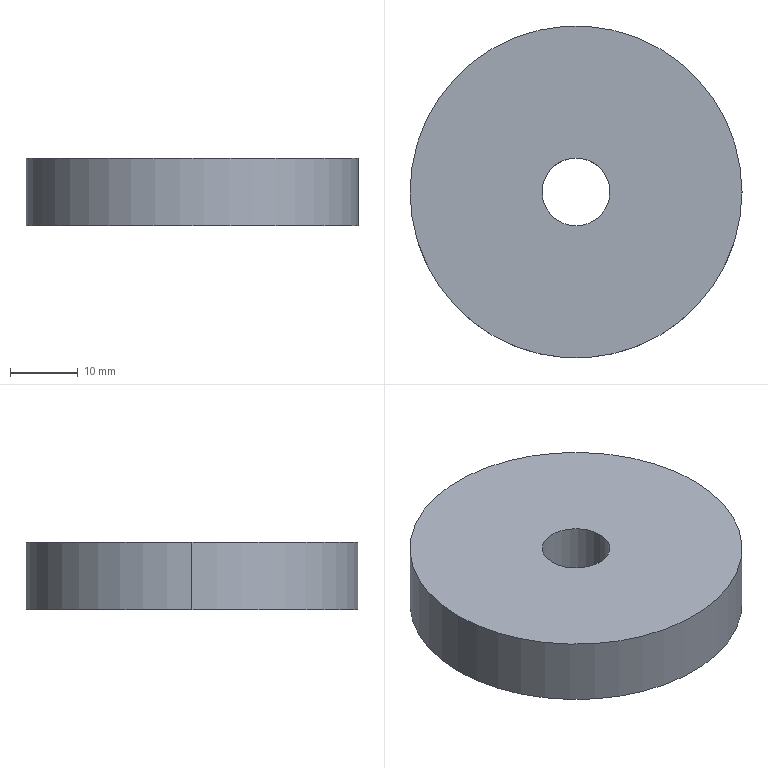Part | STEP file | Produce dryer HY-40-M-bushing clamp plate | 1 solid | 6 faces | box 49 x 49 x 10 mm | volume 18072 mm3 | cylinder 4 | plane 2 | commonest cylinder face diameters 10 x2 49 x2
STEP:
#1=CARTESIAN_POINT('',(-5.,0.,10.));
#2=VERTEX_POINT('',#1);
#3=CARTESIAN_POINT('',(5.,0.,10.));
#4=VERTEX_POINT('',#3);
#5=CARTESIAN_POINT('',(0.,0.,10.));
#6=DIRECTION('',(0.,0.,1.));
#7=DIRECTION('',(1.,0.,0.));
#8=AXIS2_PLACEMENT_3D('',#5,#6,#7);
#9=CIRCLE('',#8,5.);
#10=EDGE_CURVE('',#2,#4,#9,.T.);
#11=ORIENTED_EDGE('',*,*,#10,.T.);
#12=CARTESIAN_POINT('',(5.,0.,0.));
#13=VERTEX_POINT('',#12);
#14=CARTESIAN_POINT('',(5.,0.,10.));
#15=DIRECTION('',(0.,0.,-1.));
#16=VECTOR('',#15,1000.);
#17=LINE('',#14,#16);
#18=EDGE_CURVE('',#4,#13,#17,.T.);
#19=ORIENTED_EDGE('',*,*,#18,.T.);
#20=CARTESIAN_POINT('',(-5.,0.,0.));
#21=VERTEX_POINT('',#20);
#22=CARTESIAN_POINT('',(0.,0.,0.));
#23=DIRECTION('',(0.,0.,1.));
#24=DIRECTION('',(1.,0.,0.));
#25=AXIS2_PLACEMENT_3D('',#22,#23,#24);
#26=CIRCLE('',#25,5.);
#27=EDGE_CURVE('',#21,#13,#26,.T.);
#28=ORIENTED_EDGE('',*,*,#27,.F.);
#29=CARTESIAN_POINT('',(-5.,0.,10.));
#30=DIRECTION('',(0.,0.,-1.));
#31=VECTOR('',#30,1000.);
#32=LINE('',#29,#31);
#33=EDGE_CURVE('',#2,#21,#32,.T.);
#34=ORIENTED_EDGE('',*,*,#33,.F.);
#35=EDGE_LOOP('',(#11,#19,#28,#34));
#36=FACE_OUTER_BOUND('',#35,.T.);
#37=CARTESIAN_POINT('',(0.,0.,10.));
#38=DIRECTION('',(0.,0.,-1.));
#39=DIRECTION('',(-1.,0.,0.));
#40=AXIS2_PLACEMENT_3D('',#37,#38,#39);
#41=CYLINDRICAL_SURFACE('',#40,5.);
#42=ADVANCED_FACE('',(#36),#41,.F.);
#43=CARTESIAN_POINT('',(24.5,0.,10.));
#44=VERTEX_POINT('',#43);
#45=CARTESIAN_POINT('',(-24.5,0.,10.));
#46=VERTEX_POINT('',#45);
#47=CARTESIAN_POINT('',(0.,0.,10.));
#48=DIRECTION('',(0.,0.,1.));
#49=DIRECTION('',(1.,0.,0.));
#50=AXIS2_PLACEMENT_3D('',#47,#48,#49);
#51=CIRCLE('',#50,24.5);
#52=EDGE_CURVE('',#44,#46,#51,.T.);
#53=ORIENTED_EDGE('',*,*,#52,.F.);
#54=CARTESIAN_POINT('',(24.5,0.,0.));
#55=VERTEX_POINT('',#54);
#56=CARTESIAN_POINT('',(24.5,0.,10.));
#57=DIRECTION('',(0.,0.,-1.));
#58=VECTOR('',#57,1000.);
#59=LINE('',#56,#58);
#60=EDGE_CURVE('',#44,#55,#59,.T.);
#61=ORIENTED_EDGE('',*,*,#60,.T.);
#62=CARTESIAN_POINT('',(-24.5,0.,0.));
#63=VERTEX_POINT('',#62);
#64=CARTESIAN_POINT('',(0.,0.,0.));
#65=DIRECTION('',(0.,0.,1.));
#66=DIRECTION('',(1.,0.,0.));
#67=AXIS2_PLACEMENT_3D('',#64,#65,#66);
#68=CIRCLE('',#67,24.5);
#69=EDGE_CURVE('',#55,#63,#68,.T.);
#70=ORIENTED_EDGE('',*,*,#69,.T.);
#71=CARTESIAN_POINT('',(-24.5,0.,10.));
#72=DIRECTION('',(0.,0.,-1.));
#73=VECTOR('',#72,1000.);
#74=LINE('',#71,#73);
#75=EDGE_CURVE('',#46,#63,#74,.T.);
#76=ORIENTED_EDGE('',*,*,#75,.F.);
#77=EDGE_LOOP('',(#53,#61,#70,#76));
#78=FACE_OUTER_BOUND('',#77,.T.);
#79=CARTESIAN_POINT('',(0.,0.,10.));
#80=DIRECTION('',(0.,0.,-1.));
#81=DIRECTION('',(-1.,0.,0.));
#82=AXIS2_PLACEMENT_3D('',#79,#80,#81);
#83=CYLINDRICAL_SURFACE('',#82,24.5);
#84=ADVANCED_FACE('',(#78),#83,.T.);
#85=CARTESIAN_POINT('',(0.,0.,10.));
#86=DIRECTION('',(0.,0.,1.));
#87=DIRECTION('',(1.,0.,0.));
#88=AXIS2_PLACEMENT_3D('',#85,#86,#87);
#89=CIRCLE('',#88,24.5);
#90=EDGE_CURVE('',#46,#44,#89,.T.);
#91=ORIENTED_EDGE('',*,*,#90,.T.);
#92=ORIENTED_EDGE('',*,*,#52,.T.);
#93=EDGE_LOOP('',(#91,#92));
#94=FACE_OUTER_BOUND('',#93,.T.);
#95=ORIENTED_EDGE('',*,*,#10,.F.);
#96=CARTESIAN_POINT('',(0.,0.,10.));
#97=DIRECTION('',(0.,0.,1.));
#98=DIRECTION('',(1.,0.,0.));
#99=AXIS2_PLACEMENT_3D('',#96,#97,#98);
#100=CIRCLE('',#99,5.);
#101=EDGE_CURVE('',#4,#2,#100,.T.);
#102=ORIENTED_EDGE('',*,*,#101,.F.);
#103=EDGE_LOOP('',(#95,#102));
#104=FACE_BOUND('',#103,.T.);
#105=CARTESIAN_POINT('',(0.,0.,10.));
#106=DIRECTION('',(0.,0.,1.));
#107=DIRECTION('',(1.,0.,0.));
#108=AXIS2_PLACEMENT_3D('',#105,#106,#107);
#109=PLANE('',#108);
#110=ADVANCED_FACE('',(#94,#104),#109,.T.);
#111=CARTESIAN_POINT('',(0.,0.,0.));
#112=DIRECTION('',(0.,0.,1.));
#113=DIRECTION('',(1.,0.,0.));
#114=AXIS2_PLACEMENT_3D('',#111,#112,#113);
#115=CIRCLE('',#114,24.5);
#116=EDGE_CURVE('',#63,#55,#115,.T.);
#117=ORIENTED_EDGE('',*,*,#116,.F.);
#118=ORIENTED_EDGE('',*,*,#69,.F.);
#119=EDGE_LOOP('',(#117,#118));
#120=FACE_OUTER_BOUND('',#119,.T.);
#121=ORIENTED_EDGE('',*,*,#27,.T.);
#122=CARTESIAN_POINT('',(0.,0.,0.));
#123=DIRECTION('',(0.,0.,1.));
#124=DIRECTION('',(1.,0.,0.));
#125=AXIS2_PLACEMENT_3D('',#122,#123,#124);
#126=CIRCLE('',#125,5.);
#127=EDGE_CURVE('',#13,#21,#126,.T.);
#128=ORIENTED_EDGE('',*,*,#127,.T.);
#129=EDGE_LOOP('',(#121,#128));
#130=FACE_BOUND('',#129,.T.);
#131=CARTESIAN_POINT('',(0.,0.,0.));
#132=DIRECTION('',(0.,0.,1.));
#133=DIRECTION('',(1.,0.,0.));
#134=AXIS2_PLACEMENT_3D('',#131,#132,#133);
#135=PLANE('',#134);
#136=ADVANCED_FACE('',(#120,#130),#135,.F.);
#137=ORIENTED_EDGE('',*,*,#60,.F.);
#138=ORIENTED_EDGE('',*,*,#90,.F.);
#139=ORIENTED_EDGE('',*,*,#75,.T.);
#140=ORIENTED_EDGE('',*,*,#116,.T.);
#141=EDGE_LOOP('',(#137,#138,#139,#140));
#142=FACE_OUTER_BOUND('',#141,.T.);
#143=CARTESIAN_POINT('',(0.,0.,10.));
#144=DIRECTION('',(0.,0.,-1.));
#145=DIRECTION('',(-1.,0.,0.));
#146=AXIS2_PLACEMENT_3D('',#143,#144,#145);
#147=CYLINDRICAL_SURFACE('',#146,24.5);
#148=ADVANCED_FACE('',(#142),#147,.T.);
#149=ORIENTED_EDGE('',*,*,#18,.F.);
#150=ORIENTED_EDGE('',*,*,#101,.T.);
#151=ORIENTED_EDGE('',*,*,#33,.T.);
#152=ORIENTED_EDGE('',*,*,#127,.F.);
#153=EDGE_LOOP('',(#149,#150,#151,#152));
#154=FACE_OUTER_BOUND('',#153,.T.);
#155=CARTESIAN_POINT('',(0.,0.,10.));
#156=DIRECTION('',(0.,0.,-1.));
#157=DIRECTION('',(-1.,0.,0.));
#158=AXIS2_PLACEMENT_3D('',#155,#156,#157);
#159=CYLINDRICAL_SURFACE('',#158,5.);
#160=ADVANCED_FACE('',(#154),#159,.F.);
#161=CLOSED_SHELL('',(#42,#84,#110,#136,#148,#160));
#162=MANIFOLD_SOLID_BREP('',#161);
#163=CARTESIAN_POINT('',(0.,0.,0.));
#164=DIRECTION('',(0.,0.,1.));
#165=DIRECTION('',(1.,0.,0.));
#166=AXIS2_PLACEMENT_3D('',#163,#164,#165);
#167=(LENGTH_UNIT()NAMED_UNIT(*)SI_UNIT(.MILLI.,.METRE.));
#168=UNCERTAINTY_MEASURE_WITH_UNIT(LENGTH_MEASURE(0.00001),#167,'','');
#169=(NAMED_UNIT(*)PLANE_ANGLE_UNIT()SI_UNIT($,.RADIAN.));
#170=(NAMED_UNIT(*)SI_UNIT($,.STERADIAN.)SOLID_ANGLE_UNIT());
#171=(GEOMETRIC_REPRESENTATION_CONTEXT(3)GLOBAL_UNCERTAINTY_ASSIGNED_CONTEXT((#168))GLOBAL_UNIT_ASSIGNED_CONTEXT((#167,#169,#170))REPRESENTATION_CONTEXT('',''));
#172=ADVANCED_BREP_SHAPE_REPRESENTATION('',(#162,#166),#171);